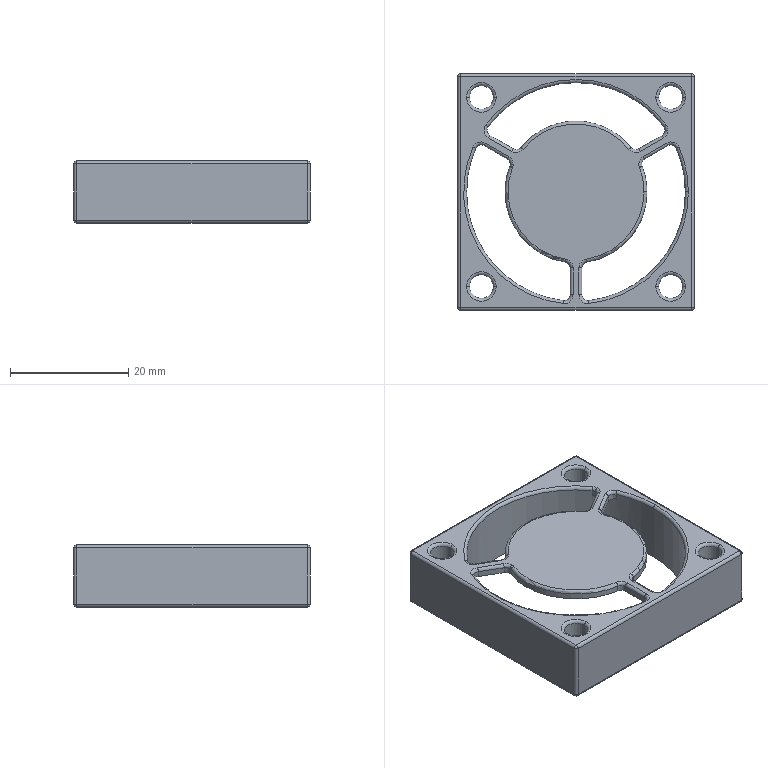Part | SolidWorks | features ICE 3, Fillet 2, Extrusion 1, Shell 1 | 1 solid | 147 faces | box 40 x 40 x 10.5 mm | volume 3410 mm3 | cylinder 76 | torus 32 | plane 31 | sphere 8 | commonest cylinder face diameters 1 x18 2 x14 3.4 x14 4 x8 5.4 x8 22.6 x4